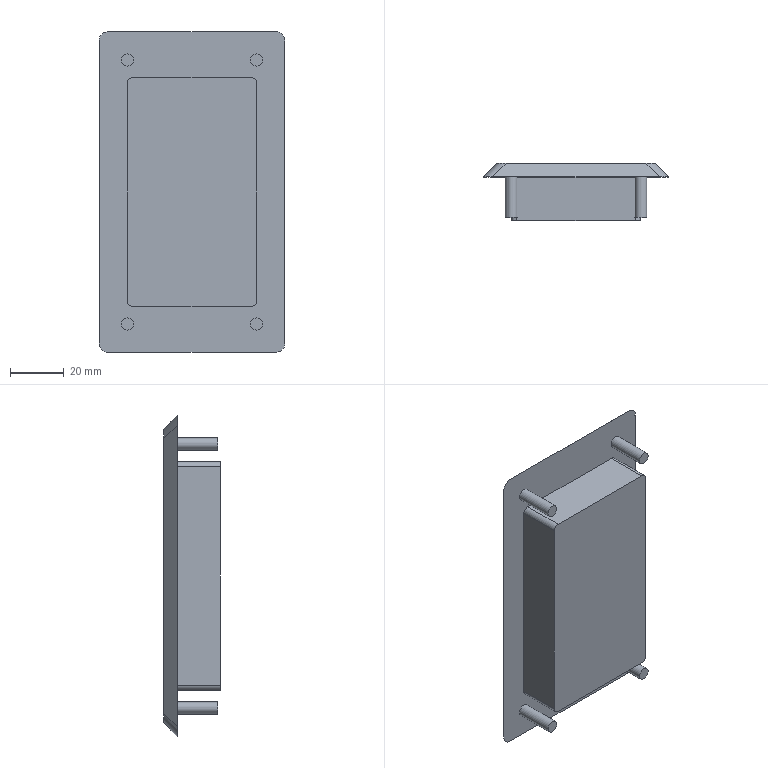Part | STEP file | 冲床-300配套压波_id522_x_t | 1 solid | 38 faces | box 69 x 21 x 119 mm | volume 44051 mm3 | plane 22 | cylinder 16 | commonest cylinder face diameters 4 x4 4.5 x4 10 x4 13 x2 20 x2
STEP:
#1=CARTESIAN_POINT('',(1655.5,280.,-353.25));
#2=VERTEX_POINT('',#1);
#3=CARTESIAN_POINT('',(1655.5,280.,-351.));
#4=DIRECTION('',(0.,-1.,0.));
#5=DIRECTION('',(0.,0.,-1.));
#6=AXIS2_PLACEMENT_3D('',#3,#4,#5);
#7=CIRCLE('',#6,2.25);
#8=EDGE_CURVE('',#2,#2,#7,.T.);
#9=ORIENTED_EDGE('',*,*,#8,.F.);
#10=EDGE_LOOP('',(#9));
#11=FACE_BOUND('',#10,.T.);
#12=CARTESIAN_POINT('',(1607.5,280.,-353.25));
#13=VERTEX_POINT('',#12);
#14=CARTESIAN_POINT('',(1607.5,280.,-351.));
#15=DIRECTION('',(0.,-1.,0.));
#16=DIRECTION('',(0.,0.,-1.));
#17=AXIS2_PLACEMENT_3D('',#14,#15,#16);
#18=CIRCLE('',#17,2.25);
#19=EDGE_CURVE('',#13,#13,#18,.T.);
#20=ORIENTED_EDGE('',*,*,#19,.F.);
#21=EDGE_LOOP('',(#20));
#22=FACE_BOUND('',#21,.T.);
#23=CARTESIAN_POINT('',(1609.5,280.,-442.5));
#24=VERTEX_POINT('',#23);
#25=CARTESIAN_POINT('',(1653.5,280.,-442.5));
#26=VERTEX_POINT('',#25);
#27=CARTESIAN_POINT('',(1467.,280.,-442.5));
#28=DIRECTION('',(1.,0.,0.));
#29=VECTOR('',#28,1.);
#30=LINE('',#27,#29);
#31=EDGE_CURVE('',#24,#26,#30,.T.);
#32=ORIENTED_EDGE('',*,*,#31,.F.);
#33=CARTESIAN_POINT('',(1607.5,280.,-440.5));
#34=VERTEX_POINT('',#33);
#35=CARTESIAN_POINT('',(1609.5,280.,-440.5));
#36=DIRECTION('',(0.,1.,0.));
#37=DIRECTION('',(0.,0.,-1.));
#38=AXIS2_PLACEMENT_3D('',#35,#36,#37);
#39=CIRCLE('',#38,2.);
#40=EDGE_CURVE('',#24,#34,#39,.T.);
#41=ORIENTED_EDGE('',*,*,#40,.T.);
#42=CARTESIAN_POINT('',(1607.5,280.,-359.5));
#43=VERTEX_POINT('',#42);
#44=CARTESIAN_POINT('',(1607.5,280.,-85.5));
#45=DIRECTION('',(0.,0.,-1.));
#46=VECTOR('',#45,1.);
#47=LINE('',#44,#46);
#48=EDGE_CURVE('',#43,#34,#47,.T.);
#49=ORIENTED_EDGE('',*,*,#48,.F.);
#50=CARTESIAN_POINT('',(1609.5,280.,-357.5));
#51=VERTEX_POINT('',#50);
#52=CARTESIAN_POINT('',(1609.5,280.,-359.5));
#53=DIRECTION('',(0.,1.,0.));
#54=DIRECTION('',(0.,0.,-1.));
#55=AXIS2_PLACEMENT_3D('',#52,#53,#54);
#56=CIRCLE('',#55,2.);
#57=EDGE_CURVE('',#43,#51,#56,.T.);
#58=ORIENTED_EDGE('',*,*,#57,.T.);
#59=CARTESIAN_POINT('',(1653.5,280.,-357.5));
#60=VERTEX_POINT('',#59);
#61=CARTESIAN_POINT('',(1467.,280.,-357.5));
#62=DIRECTION('',(-1.,0.,0.));
#63=VECTOR('',#62,1.);
#64=LINE('',#61,#63);
#65=EDGE_CURVE('',#60,#51,#64,.T.);
#66=ORIENTED_EDGE('',*,*,#65,.F.);
#67=CARTESIAN_POINT('',(1655.5,280.,-359.5));
#68=VERTEX_POINT('',#67);
#69=CARTESIAN_POINT('',(1653.5,280.,-359.5));
#70=DIRECTION('',(0.,1.,0.));
#71=DIRECTION('',(0.,0.,-1.));
#72=AXIS2_PLACEMENT_3D('',#69,#70,#71);
#73=CIRCLE('',#72,2.);
#74=EDGE_CURVE('',#60,#68,#73,.T.);
#75=ORIENTED_EDGE('',*,*,#74,.T.);
#76=CARTESIAN_POINT('',(1655.5,280.,-440.5));
#77=VERTEX_POINT('',#76);
#78=CARTESIAN_POINT('',(1655.5,280.,-85.5));
#79=DIRECTION('',(0.,0.,1.));
#80=VECTOR('',#79,1.);
#81=LINE('',#78,#80);
#82=EDGE_CURVE('',#77,#68,#81,.T.);
#83=ORIENTED_EDGE('',*,*,#82,.F.);
#84=CARTESIAN_POINT('',(1653.5,280.,-440.5));
#85=DIRECTION('',(0.,1.,0.));
#86=DIRECTION('',(0.,0.,-1.));
#87=AXIS2_PLACEMENT_3D('',#84,#85,#86);
#88=CIRCLE('',#87,2.);
#89=EDGE_CURVE('',#77,#26,#88,.T.);
#90=ORIENTED_EDGE('',*,*,#89,.T.);
#91=EDGE_LOOP('',(#32,#41,#49,#58,#66,#75,#83,#90));
#92=FACE_BOUND('',#91,.T.);
#93=CARTESIAN_POINT('',(1666.,280.,-344.036));
#94=VERTEX_POINT('',#93);
#95=CARTESIAN_POINT('',(1666.,280.,-455.964));
#96=VERTEX_POINT('',#95);
#97=CARTESIAN_POINT('',(1666.,280.,-459.5));
#98=DIRECTION('',(0.,0.,-1.));
#99=VECTOR('',#98,1.);
#100=LINE('',#97,#99);
#101=EDGE_CURVE('',#94,#96,#100,.T.);
#102=ORIENTED_EDGE('',*,*,#101,.F.);
#103=CARTESIAN_POINT('',(1662.464,280.,-340.5));
#104=VERTEX_POINT('',#103);
#105=CARTESIAN_POINT('',(1658.929,280.,-347.571));
#106=DIRECTION('',(0.,-1.,0.));
#107=DIRECTION('',(0.7071,0.,0.7071));
#108=AXIS2_PLACEMENT_3D('',#105,#106,#107);
#109=ELLIPSE('',#108,8.66,5.);
#110=EDGE_CURVE('',#94,#104,#109,.T.);
#111=ORIENTED_EDGE('',*,*,#110,.T.);
#112=CARTESIAN_POINT('',(1600.536,280.,-340.5));
#113=VERTEX_POINT('',#112);
#114=CARTESIAN_POINT('',(1666.,280.,-340.5));
#115=DIRECTION('',(1.,0.,0.));
#116=VECTOR('',#115,1.);
#117=LINE('',#114,#116);
#118=EDGE_CURVE('',#113,#104,#117,.T.);
#119=ORIENTED_EDGE('',*,*,#118,.F.);
#120=CARTESIAN_POINT('',(1597.,280.,-344.036));
#121=VERTEX_POINT('',#120);
#122=CARTESIAN_POINT('',(1604.071,280.,-347.571));
#123=DIRECTION('',(0.,-1.,0.));
#124=DIRECTION('',(-0.7071,0.,0.7071));
#125=AXIS2_PLACEMENT_3D('',#122,#123,#124);
#126=ELLIPSE('',#125,8.66,5.);
#127=EDGE_CURVE('',#113,#121,#126,.T.);
#128=ORIENTED_EDGE('',*,*,#127,.T.);
#129=CARTESIAN_POINT('',(1597.,280.,-455.964));
#130=VERTEX_POINT('',#129);
#131=CARTESIAN_POINT('',(1597.,280.,-340.5));
#132=DIRECTION('',(0.,0.,1.));
#133=VECTOR('',#132,1.);
#134=LINE('',#131,#133);
#135=EDGE_CURVE('',#130,#121,#134,.T.);
#136=ORIENTED_EDGE('',*,*,#135,.F.);
#137=CARTESIAN_POINT('',(1600.536,280.,-459.5));
#138=VERTEX_POINT('',#137);
#139=CARTESIAN_POINT('',(1604.071,280.,-452.429));
#140=DIRECTION('',(0.,-1.,0.));
#141=DIRECTION('',(-0.7071,0.,-0.7071));
#142=AXIS2_PLACEMENT_3D('',#139,#140,#141);
#143=ELLIPSE('',#142,8.66,5.);
#144=EDGE_CURVE('',#130,#138,#143,.T.);
#145=ORIENTED_EDGE('',*,*,#144,.T.);
#146=CARTESIAN_POINT('',(1662.464,280.,-459.5));
#147=VERTEX_POINT('',#146);
#148=CARTESIAN_POINT('',(1597.,280.,-459.5));
#149=DIRECTION('',(-1.,0.,0.));
#150=VECTOR('',#149,1.);
#151=LINE('',#148,#150);
#152=EDGE_CURVE('',#147,#138,#151,.T.);
#153=ORIENTED_EDGE('',*,*,#152,.F.);
#154=CARTESIAN_POINT('',(1658.929,280.,-452.429));
#155=DIRECTION('',(0.,-1.,0.));
#156=DIRECTION('',(0.7071,0.,-0.7071));
#157=AXIS2_PLACEMENT_3D('',#154,#155,#156);
#158=ELLIPSE('',#157,8.66,5.);
#159=EDGE_CURVE('',#147,#96,#158,.T.);
#160=ORIENTED_EDGE('',*,*,#159,.T.);
#161=EDGE_LOOP('',(#102,#111,#119,#128,#136,#145,#153,#160));
#162=FACE_BOUND('',#161,.T.);
#163=CARTESIAN_POINT('',(1655.5,280.,-451.25));
#164=VERTEX_POINT('',#163);
#165=CARTESIAN_POINT('',(1655.5,280.,-449.));
#166=DIRECTION('',(0.,-1.,0.));
#167=DIRECTION('',(0.,0.,-1.));
#168=AXIS2_PLACEMENT_3D('',#165,#166,#167);
#169=CIRCLE('',#168,2.25);
#170=EDGE_CURVE('',#164,#164,#169,.T.);
#171=ORIENTED_EDGE('',*,*,#170,.F.);
#172=EDGE_LOOP('',(#171));
#173=FACE_BOUND('',#172,.T.);
#174=CARTESIAN_POINT('',(1607.5,280.,-451.25));
#175=VERTEX_POINT('',#174);
#176=CARTESIAN_POINT('',(1607.5,280.,-449.));
#177=DIRECTION('',(0.,1.,0.));
#178=DIRECTION('',(0.,0.,-1.));
#179=AXIS2_PLACEMENT_3D('',#176,#177,#178);
#180=CIRCLE('',#179,2.25);
#181=EDGE_CURVE('',#175,#175,#180,.T.);
#182=ORIENTED_EDGE('',*,*,#181,.T.);
#183=EDGE_LOOP('',(#182));
#184=FACE_BOUND('',#183,.T.);
#185=CARTESIAN_POINT('',(1467.,280.,-85.5));
#186=DIRECTION('',(0.,1.,0.));
#187=DIRECTION('',(0.,0.,-1.));
#188=AXIS2_PLACEMENT_3D('',#185,#186,#187);
#189=PLANE('',#188);
#190=ADVANCED_FACE('',(#11,#22,#92,#162,#173,#184),#189,.F.);
#191=CARTESIAN_POINT('',(1648.5,285.,-359.5));
#192=VERTEX_POINT('',#191);
#193=CARTESIAN_POINT('',(1655.,285.,-366.));
#194=VERTEX_POINT('',#193);
#195=CARTESIAN_POINT('',(1648.5,285.,-366.));
#196=DIRECTION('',(0.,1.,0.));
#197=DIRECTION('',(0.,0.,-1.));
#198=AXIS2_PLACEMENT_3D('',#195,#196,#197);
#199=CIRCLE('',#198,6.5);
#200=EDGE_CURVE('',#192,#194,#199,.T.);
#201=ORIENTED_EDGE('',*,*,#200,.F.);
#202=CARTESIAN_POINT('',(1627.,285.,-359.5));
#203=VERTEX_POINT('',#202);
#204=CARTESIAN_POINT('',(1467.,285.,-359.5));
#205=DIRECTION('',(-1.,0.,0.));
#206=VECTOR('',#205,1.);
#207=LINE('',#204,#206);
#208=EDGE_CURVE('',#192,#203,#207,.T.);
#209=ORIENTED_EDGE('',*,*,#208,.T.);
#210=CARTESIAN_POINT('',(1627.,285.,-440.5));
#211=VERTEX_POINT('',#210);
#212=CARTESIAN_POINT('',(1627.,285.,-85.5));
#213=DIRECTION('',(0.,0.,-1.));
#214=VECTOR('',#213,1.);
#215=LINE('',#212,#214);
#216=EDGE_CURVE('',#203,#211,#215,.T.);
#217=ORIENTED_EDGE('',*,*,#216,.T.);
#218=CARTESIAN_POINT('',(1648.5,285.,-440.5));
#219=VERTEX_POINT('',#218);
#220=CARTESIAN_POINT('',(1467.,285.,-440.5));
#221=DIRECTION('',(1.,0.,0.));
#222=VECTOR('',#221,1.);
#223=LINE('',#220,#222);
#224=EDGE_CURVE('',#211,#219,#223,.T.);
#225=ORIENTED_EDGE('',*,*,#224,.T.);
#226=CARTESIAN_POINT('',(1655.,285.,-434.));
#227=VERTEX_POINT('',#226);
#228=CARTESIAN_POINT('',(1648.5,285.,-434.));
#229=DIRECTION('',(0.,1.,0.));
#230=DIRECTION('',(0.,0.,-1.));
#231=AXIS2_PLACEMENT_3D('',#228,#229,#230);
#232=CIRCLE('',#231,6.5);
#233=EDGE_CURVE('',#227,#219,#232,.T.);
#234=ORIENTED_EDGE('',*,*,#233,.F.);
#235=CARTESIAN_POINT('',(1655.,285.,-85.5));
#236=DIRECTION('',(0.,0.,1.));
#237=VECTOR('',#236,1.);
#238=LINE('',#235,#237);
#239=EDGE_CURVE('',#227,#194,#238,.T.);
#240=ORIENTED_EDGE('',*,*,#239,.T.);
#241=EDGE_LOOP('',(#201,#209,#217,#225,#234,#240));
#242=FACE_BOUND('',#241,.T.);
#243=CARTESIAN_POINT('',(1657.464,285.,-454.5));
#244=VERTEX_POINT('',#243);
#245=CARTESIAN_POINT('',(1605.536,285.,-454.5));
#246=VERTEX_POINT('',#245);
#247=CARTESIAN_POINT('',(1661.,285.,-454.5));
#248=DIRECTION('',(-1.,0.,0.));
#249=VECTOR('',#248,1.);
#250=LINE('',#247,#249);
#251=EDGE_CURVE('',#244,#246,#250,.T.);
#252=ORIENTED_EDGE('',*,*,#251,.T.);
#253=CARTESIAN_POINT('',(1602.,285.,-450.964));
#254=VERTEX_POINT('',#253);
#255=CARTESIAN_POINT('',(1609.071,285.,-447.429));
#256=DIRECTION('',(0.,1.,0.));
#257=DIRECTION('',(-0.7071,0.,-0.7071));
#258=AXIS2_PLACEMENT_3D('',#255,#256,#257);
#259=ELLIPSE('',#258,8.66,5.);
#260=EDGE_CURVE('',#246,#254,#259,.T.);
#261=ORIENTED_EDGE('',*,*,#260,.T.);
#262=CARTESIAN_POINT('',(1602.,285.,-349.036));
#263=VERTEX_POINT('',#262);
#264=CARTESIAN_POINT('',(1602.,285.,-454.5));
#265=DIRECTION('',(0.,0.,1.));
#266=VECTOR('',#265,1.);
#267=LINE('',#264,#266);
#268=EDGE_CURVE('',#254,#263,#267,.T.);
#269=ORIENTED_EDGE('',*,*,#268,.T.);
#270=CARTESIAN_POINT('',(1605.536,285.,-345.5));
#271=VERTEX_POINT('',#270);
#272=CARTESIAN_POINT('',(1609.071,285.,-352.571));
#273=DIRECTION('',(0.,1.,0.));
#274=DIRECTION('',(-0.7071,0.,0.7071));
#275=AXIS2_PLACEMENT_3D('',#272,#273,#274);
#276=ELLIPSE('',#275,8.66,5.);
#277=EDGE_CURVE('',#263,#271,#276,.T.);
#278=ORIENTED_EDGE('',*,*,#277,.T.);
#279=CARTESIAN_POINT('',(1657.464,285.,-345.5));
#280=VERTEX_POINT('',#279);
#281=CARTESIAN_POINT('',(1602.,285.,-345.5));
#282=DIRECTION('',(1.,0.,0.));
#283=VECTOR('',#282,1.);
#284=LINE('',#281,#283);
#285=EDGE_CURVE('',#271,#280,#284,.T.);
#286=ORIENTED_EDGE('',*,*,#285,.T.);
#287=CARTESIAN_POINT('',(1661.,285.,-349.036));
#288=VERTEX_POINT('',#287);
#289=CARTESIAN_POINT('',(1653.929,285.,-352.571));
#290=DIRECTION('',(0.,1.,0.));
#291=DIRECTION('',(0.7071,0.,0.7071));
#292=AXIS2_PLACEMENT_3D('',#289,#290,#291);
#293=ELLIPSE('',#292,8.66,5.);
#294=EDGE_CURVE('',#280,#288,#293,.T.);
#295=ORIENTED_EDGE('',*,*,#294,.T.);
#296=CARTESIAN_POINT('',(1661.,285.,-450.964));
#297=VERTEX_POINT('',#296);
#298=CARTESIAN_POINT('',(1661.,285.,-345.5));
#299=DIRECTION('',(0.,0.,-1.));
#300=VECTOR('',#299,1.);
#301=LINE('',#298,#300);
#302=EDGE_CURVE('',#288,#297,#301,.T.);
#303=ORIENTED_EDGE('',*,*,#302,.T.);
#304=CARTESIAN_POINT('',(1653.929,285.,-447.429));
#305=DIRECTION('',(0.,1.,0.));
#306=DIRECTION('',(0.7071,0.,-0.7071));
#307=AXIS2_PLACEMENT_3D('',#304,#305,#306);
#308=ELLIPSE('',#307,8.66,5.);
#309=EDGE_CURVE('',#297,#244,#308,.T.);
#310=ORIENTED_EDGE('',*,*,#309,.T.);
#311=EDGE_LOOP('',(#252,#261,#269,#278,#286,#295,#303,#310));
#312=FACE_BOUND('',#311,.T.);
#313=CARTESIAN_POINT('',(1467.,285.,-85.5));
#314=DIRECTION('',(0.,1.,0.));
#315=DIRECTION('',(0.,0.,-1.));
#316=AXIS2_PLACEMENT_3D('',#313,#314,#315);
#317=PLANE('',#316);
#318=ADVANCED_FACE('',(#242,#312),#317,.T.);
#319=CARTESIAN_POINT('',(1619.,266.5,-440.5));
#320=VERTEX_POINT('',#319);
#321=CARTESIAN_POINT('',(1648.5,266.5,-440.5));
#322=VERTEX_POINT('',#321);
#323=CARTESIAN_POINT('',(1467.,266.5,-440.5));
#324=DIRECTION('',(1.,0.,0.));
#325=VECTOR('',#324,1.);
#326=LINE('',#323,#325);
#327=EDGE_CURVE('',#320,#322,#326,.T.);
#328=ORIENTED_EDGE('',*,*,#327,.T.);
#329=CARTESIAN_POINT('',(1648.5,254.,-440.5));
#330=DIRECTION('',(0.,-1.,0.));
#331=VECTOR('',#330,1.);
#332=LINE('',#329,#331);
#333=EDGE_CURVE('',#219,#322,#332,.T.);
#334=ORIENTED_EDGE('',*,*,#333,.F.);
#335=ORIENTED_EDGE('',*,*,#224,.F.);
#336=CARTESIAN_POINT('',(1627.,278.5,-440.5));
#337=VERTEX_POINT('',#336);
#338=CARTESIAN_POINT('',(1627.,254.,-440.5));
#339=DIRECTION('',(0.,1.,0.));
#340=VECTOR('',#339,1.);
#341=LINE('',#338,#340);
#342=EDGE_CURVE('',#337,#211,#341,.T.);
#343=ORIENTED_EDGE('',*,*,#342,.F.);
#344=CARTESIAN_POINT('',(1619.,278.5,-440.5));
#345=VERTEX_POINT('',#344);
#346=CARTESIAN_POINT('',(1655.,278.5,-440.5));
#347=DIRECTION('',(-1.,0.,0.));
#348=VECTOR('',#347,1.);
#349=LINE('',#346,#348);
#350=EDGE_CURVE('',#337,#345,#349,.T.);
#351=ORIENTED_EDGE('',*,*,#350,.T.);
#352=CARTESIAN_POINT('',(1619.,254.,-440.5));
#353=DIRECTION('',(0.,-1.,0.));
#354=VECTOR('',#353,1.);
#355=LINE('',#352,#354);
#356=EDGE_CURVE('',#345,#320,#355,.T.);
#357=ORIENTED_EDGE('',*,*,#356,.T.);
#358=EDGE_LOOP('',(#328,#334,#335,#343,#351,#357));
#359=FACE_OUTER_BOUND('',#358,.T.);
#360=CARTESIAN_POINT('',(1655.,254.,-440.5));
#361=DIRECTION('',(0.,0.,1.));
#362=DIRECTION('',(1.,0.,0.));
#363=AXIS2_PLACEMENT_3D('',#360,#361,#362);
#364=PLANE('',#363);
#365=ADVANCED_FACE('',(#359),#364,.T.);
#366=CARTESIAN_POINT('',(1655.,266.5,-434.));
#367=VERTEX_POINT('',#366);
#368=CARTESIAN_POINT('',(1655.,254.,-434.));
#369=DIRECTION('',(0.,-1.,0.));
#370=VECTOR('',#369,1.);
#371=LINE('',#368,#370);
#372=EDGE_CURVE('',#227,#367,#371,.T.);
#373=ORIENTED_EDGE('',*,*,#372,.T.);
#374=CARTESIAN_POINT('',(1655.,266.5,-366.));
#375=VERTEX_POINT('',#374);
#376=CARTESIAN_POINT('',(1655.,266.5,-85.5));
#377=DIRECTION('',(0.,0.,1.));
#378=VECTOR('',#377,1.);
#379=LINE('',#376,#378);
#380=EDGE_CURVE('',#367,#375,#379,.T.);
#381=ORIENTED_EDGE('',*,*,#380,.T.);
#382=CARTESIAN_POINT('',(1655.,254.,-366.));
#383=DIRECTION('',(0.,-1.,0.));
#384=VECTOR('',#383,1.);
#385=LINE('',#382,#384);
#386=EDGE_CURVE('',#194,#375,#385,.T.);
#387=ORIENTED_EDGE('',*,*,#386,.F.);
#388=ORIENTED_EDGE('',*,*,#239,.F.);
#389=EDGE_LOOP('',(#373,#381,#387,#388));
#390=FACE_OUTER_BOUND('',#389,.T.);
#391=CARTESIAN_POINT('',(1655.,254.,-359.5));
#392=DIRECTION('',(-1.,0.,0.));
#393=DIRECTION('',(0.,0.,1.));
#394=AXIS2_PLACEMENT_3D('',#391,#392,#393);
#395=PLANE('',#394);
#396=ADVANCED_FACE('',(#390),#395,.T.);
#397=CARTESIAN_POINT('',(1619.,278.5,-359.5));
#398=VERTEX_POINT('',#397);
#399=CARTESIAN_POINT('',(1627.,278.5,-359.5));
#400=VERTEX_POINT('',#399);
#401=CARTESIAN_POINT('',(1627.,278.5,-359.5));
#402=DIRECTION('',(1.,0.,0.));
#403=VECTOR('',#402,1.);
#404=LINE('',#401,#403);
#405=EDGE_CURVE('',#398,#400,#404,.T.);
#406=ORIENTED_EDGE('',*,*,#405,.T.);
#407=CARTESIAN_POINT('',(1627.,279.,-359.5));
#408=DIRECTION('',(0.,1.,0.));
#409=VECTOR('',#408,1.);
#410=LINE('',#407,#409);
#411=EDGE_CURVE('',#400,#203,#410,.T.);
#412=ORIENTED_EDGE('',*,*,#411,.T.);
#413=ORIENTED_EDGE('',*,*,#208,.F.);
#414=CARTESIAN_POINT('',(1648.5,266.5,-359.5));
#415=VERTEX_POINT('',#414);
#416=CARTESIAN_POINT('',(1648.5,254.,-359.5));
#417=DIRECTION('',(0.,-1.,0.));
#418=VECTOR('',#417,1.);
#419=LINE('',#416,#418);
#420=EDGE_CURVE('',#192,#415,#419,.T.);
#421=ORIENTED_EDGE('',*,*,#420,.T.);
#422=CARTESIAN_POINT('',(1619.,266.5,-359.5));
#423=VERTEX_POINT('',#422);
#424=CARTESIAN_POINT('',(1467.,266.5,-359.5));
#425=DIRECTION('',(-1.,0.,0.));
#426=VECTOR('',#425,1.);
#427=LINE('',#424,#426);
#428=EDGE_CURVE('',#415,#423,#427,.T.);
#429=ORIENTED_EDGE('',*,*,#428,.T.);
#430=CARTESIAN_POINT('',(1619.,254.,-359.5));
#431=DIRECTION('',(0.,1.,0.));
#432=VECTOR('',#431,1.);
#433=LINE('',#430,#432);
#434=EDGE_CURVE('',#423,#398,#433,.T.);
#435=ORIENTED_EDGE('',*,*,#434,.T.);
#436=EDGE_LOOP('',(#406,#412,#413,#421,#429,#435));
#437=FACE_OUTER_BOUND('',#436,.T.);
#438=CARTESIAN_POINT('',(1627.,254.,-359.5));
#439=DIRECTION('',(0.,0.,-1.));
#440=DIRECTION('',(-1.,0.,0.));
#441=AXIS2_PLACEMENT_3D('',#438,#439,#440);
#442=PLANE('',#441);
#443=ADVANCED_FACE('',(#437),#442,.T.);
#444=ORIENTED_EDGE('',*,*,#342,.T.);
#445=ORIENTED_EDGE('',*,*,#216,.F.);
#446=ORIENTED_EDGE('',*,*,#411,.F.);
#447=CARTESIAN_POINT('',(1627.,278.5,-359.5));
#448=DIRECTION('',(0.,0.,-1.));
#449=VECTOR('',#448,1.);
#450=LINE('',#447,#449);
#451=EDGE_CURVE('',#400,#337,#450,.T.);
#452=ORIENTED_EDGE('',*,*,#451,.T.);
#453=EDGE_LOOP('',(#444,#445,#446,#452));
#454=FACE_OUTER_BOUND('',#453,.T.);
#455=CARTESIAN_POINT('',(1627.,279.,-359.5));
#456=DIRECTION('',(-1.,0.,0.));
#457=DIRECTION('',(0.,0.,1.));
#458=AXIS2_PLACEMENT_3D('',#455,#456,#457);
#459=PLANE('',#458);
#460=ADVANCED_FACE('',(#454),#459,.F.);
#461=CARTESIAN_POINT('',(1609.,278.5,-369.5));
#462=VERTEX_POINT('',#461);
#463=CARTESIAN_POINT('',(1609.,278.5,-430.5));
#464=VERTEX_POINT('',#463);
#465=CARTESIAN_POINT('',(1609.,278.5,-443.));
#466=DIRECTION('',(0.,0.,-1.));
#467=VECTOR('',#466,1.);
#468=LINE('',#465,#467);
#469=EDGE_CURVE('',#462,#464,#468,.T.);
#470=ORIENTED_EDGE('',*,*,#469,.F.);
#471=CARTESIAN_POINT('',(1609.,266.5,-369.5));
#472=VERTEX_POINT('',#471);
#473=CARTESIAN_POINT('',(1609.,265.,-369.5));
#474=DIRECTION('',(0.,-1.,0.));
#475=VECTOR('',#474,1.);
#476=LINE('',#473,#475);
#477=EDGE_CURVE('',#462,#472,#476,.T.);
#478=ORIENTED_EDGE('',*,*,#477,.T.);
#479=CARTESIAN_POINT('',(1609.,266.5,-430.5));
#480=VERTEX_POINT('',#479);
#481=CARTESIAN_POINT('',(1609.,266.5,-443.));
#482=DIRECTION('',(0.,0.,-1.));
#483=VECTOR('',#482,1.);
#484=LINE('',#481,#483);
#485=EDGE_CURVE('',#472,#480,#484,.T.);
#486=ORIENTED_EDGE('',*,*,#485,.T.);
#487=CARTESIAN_POINT('',(1609.,265.,-430.5));
#488=DIRECTION('',(0.,1.,0.));
#489=VECTOR('',#488,1.);
#490=LINE('',#487,#489);
#491=EDGE_CURVE('',#480,#464,#490,.T.);
#492=ORIENTED_EDGE('',*,*,#491,.T.);
#493=EDGE_LOOP('',(#470,#478,#486,#492));
#494=FACE_OUTER_BOUND('',#493,.T.);
#495=CARTESIAN_POINT('',(1609.,265.,-443.));
#496=DIRECTION('',(1.,0.,0.));
#497=DIRECTION('',(0.,0.,-1.));
#498=AXIS2_PLACEMENT_3D('',#495,#496,#497);
#499=PLANE('',#498);
#500=ADVANCED_FACE('',(#494),#499,.T.);
#501=ORIENTED_EDGE('',*,*,#485,.F.);
#502=CARTESIAN_POINT('',(1619.,266.5,-369.5));
#503=DIRECTION('',(0.,1.,0.));
#504=DIRECTION('',(0.,0.,1.));
#505=AXIS2_PLACEMENT_3D('',#502,#503,#504);
#506=CIRCLE('',#505,10.);
#507=EDGE_CURVE('',#472,#423,#506,.T.);
#508=ORIENTED_EDGE('',*,*,#507,.T.);
#509=ORIENTED_EDGE('',*,*,#428,.F.);
#510=CARTESIAN_POINT('',(1648.5,266.5,-366.));
#511=DIRECTION('',(0.,-1.,0.));
#512=DIRECTION('',(0.,0.,1.));
#513=AXIS2_PLACEMENT_3D('',#510,#511,#512);
#514=CIRCLE('',#513,6.5);
#515=EDGE_CURVE('',#375,#415,#514,.T.);
#516=ORIENTED_EDGE('',*,*,#515,.F.);
#517=ORIENTED_EDGE('',*,*,#380,.F.);
#518=CARTESIAN_POINT('',(1648.5,266.5,-434.));
#519=DIRECTION('',(0.,-1.,0.));
#520=DIRECTION('',(0.,0.,1.));
#521=AXIS2_PLACEMENT_3D('',#518,#519,#520);
#522=CIRCLE('',#521,6.5);
#523=EDGE_CURVE('',#322,#367,#522,.T.);
#524=ORIENTED_EDGE('',*,*,#523,.F.);
#525=ORIENTED_EDGE('',*,*,#327,.F.);
#526=CARTESIAN_POINT('',(1619.,266.5,-430.5));
#527=DIRECTION('',(0.,1.,0.));
#528=DIRECTION('',(0.,0.,1.));
#529=AXIS2_PLACEMENT_3D('',#526,#527,#528);
#530=CIRCLE('',#529,10.);
#531=EDGE_CURVE('',#320,#480,#530,.T.);
#532=ORIENTED_EDGE('',*,*,#531,.T.);
#533=EDGE_LOOP('',(#501,#508,#509,#516,#517,#524,#525,#532));
#534=FACE_OUTER_BOUND('',#533,.T.);
#535=CARTESIAN_POINT('',(1467.,266.5,-85.5));
#536=DIRECTION('',(0.,-1.,0.));
#537=DIRECTION('',(0.,0.,1.));
#538=AXIS2_PLACEMENT_3D('',#535,#536,#537);
#539=PLANE('',#538);
#540=ADVANCED_FACE('',(#534),#539,.F.);
#541=ORIENTED_EDGE('',*,*,#350,.F.);
#542=ORIENTED_EDGE('',*,*,#451,.F.);
#543=ORIENTED_EDGE('',*,*,#405,.F.);
#544=CARTESIAN_POINT('',(1619.,278.5,-369.5));
#545=DIRECTION('',(0.,-1.,0.));
#546=DIRECTION('',(0.,0.,1.));
#547=AXIS2_PLACEMENT_3D('',#544,#545,#546);
#548=CIRCLE('',#547,10.);
#549=EDGE_CURVE('',#398,#462,#548,.T.);
#550=ORIENTED_EDGE('',*,*,#549,.T.);
#551=ORIENTED_EDGE('',*,*,#469,.T.);
#552=CARTESIAN_POINT('',(1619.,278.5,-430.5));
#553=DIRECTION('',(0.,-1.,0.));
#554=DIRECTION('',(0.,0.,1.));
#555=AXIS2_PLACEMENT_3D('',#552,#553,#554);
#556=CIRCLE('',#555,10.);
#557=EDGE_CURVE('',#464,#345,#556,.T.);
#558=ORIENTED_EDGE('',*,*,#557,.T.);
#559=EDGE_LOOP('',(#541,#542,#543,#550,#551,#558));
#560=FACE_OUTER_BOUND('',#559,.T.);
#561=CARTESIAN_POINT('',(1467.,278.5,-85.5));
#562=DIRECTION('',(0.,-1.,0.));
#563=DIRECTION('',(0.,0.,1.));
#564=AXIS2_PLACEMENT_3D('',#561,#562,#563);
#565=PLANE('',#564);
#566=ADVANCED_FACE('',(#560),#565,.T.);
#567=ORIENTED_EDGE('',*,*,#523,.T.);
#568=ORIENTED_EDGE('',*,*,#372,.F.);
#569=ORIENTED_EDGE('',*,*,#233,.T.);
#570=ORIENTED_EDGE('',*,*,#333,.T.);
#571=EDGE_LOOP('',(#567,#568,#569,#570));
#572=FACE_OUTER_BOUND('',#571,.T.);
#573=CARTESIAN_POINT('',(1648.5,254.,-434.));
#574=DIRECTION('',(0.,1.,0.));
#575=DIRECTION('',(0.,0.,-1.));
#576=AXIS2_PLACEMENT_3D('',#573,#574,#575);
#577=CYLINDRICAL_SURFACE('',#576,6.5);
#578=ADVANCED_FACE('',(#572),#577,.F.);
#579=ORIENTED_EDGE('',*,*,#515,.T.);
#580=ORIENTED_EDGE('',*,*,#420,.F.);
#581=ORIENTED_EDGE('',*,*,#200,.T.);
#582=ORIENTED_EDGE('',*,*,#386,.T.);
#583=EDGE_LOOP('',(#579,#580,#581,#582));
#584=FACE_OUTER_BOUND('',#583,.T.);
#585=CARTESIAN_POINT('',(1648.5,254.,-366.));
#586=DIRECTION('',(0.,1.,0.));
#587=DIRECTION('',(0.,0.,-1.));
#588=AXIS2_PLACEMENT_3D('',#585,#586,#587);
#589=CYLINDRICAL_SURFACE('',#588,6.5);
#590=ADVANCED_FACE('',(#584),#589,.F.);
#591=ORIENTED_EDGE('',*,*,#118,.T.);
#592=CARTESIAN_POINT('',(1593.976,348.488,-408.988));
#593=DIRECTION('',(-0.5774,0.5774,-0.5774));
#594=VECTOR('',#593,1.);
#595=LINE('',#592,#594);
#596=EDGE_CURVE('',#104,#280,#595,.T.);
#597=ORIENTED_EDGE('',*,*,#596,.T.);
#598=ORIENTED_EDGE('',*,*,#285,.F.);
#599=CARTESIAN_POINT('',(1559.357,238.821,-299.321));
#600=DIRECTION('',(-0.5774,-0.5774,0.5774));
#601=VECTOR('',#600,1.);
#602=LINE('',#599,#601);
#603=EDGE_CURVE('',#271,#113,#602,.T.);
#604=ORIENTED_EDGE('',*,*,#603,.T.);
#605=EDGE_LOOP('',(#591,#597,#598,#604));
#606=FACE_OUTER_BOUND('',#605,.T.);
#607=CARTESIAN_POINT('',(1467.,285.,-345.5));
#608=DIRECTION('',(0.,0.7071,0.7071));
#609=DIRECTION('',(1.,0.,0.));
#610=AXIS2_PLACEMENT_3D('',#607,#608,#609);
#611=PLANE('',#610);
#612=ADVANCED_FACE('',(#606),#611,.T.);
#613=ORIENTED_EDGE('',*,*,#302,.F.);
#614=CARTESIAN_POINT('',(1748.845,197.155,-261.19));
#615=DIRECTION('',(0.5774,-0.5774,0.5774));
#616=VECTOR('',#615,1.);
#617=LINE('',#614,#616);
#618=EDGE_CURVE('',#288,#94,#617,.T.);
#619=ORIENTED_EDGE('',*,*,#618,.T.);
#620=ORIENTED_EDGE('',*,*,#101,.T.);
#621=CARTESIAN_POINT('',(1539.179,406.821,-329.143));
#622=DIRECTION('',(-0.5774,0.5774,0.5774));
#623=VECTOR('',#622,1.);
#624=LINE('',#621,#623);
#625=EDGE_CURVE('',#96,#297,#624,.T.);
#626=ORIENTED_EDGE('',*,*,#625,.T.);
#627=EDGE_LOOP('',(#613,#619,#620,#626));
#628=FACE_OUTER_BOUND('',#627,.T.);
#629=CARTESIAN_POINT('',(1661.,285.,-85.5));
#630=DIRECTION('',(0.7071,0.7071,0.));
#631=DIRECTION('',(0.,0.,-1.));
#632=AXIS2_PLACEMENT_3D('',#629,#630,#631);
#633=PLANE('',#632);
#634=ADVANCED_FACE('',(#628),#633,.T.);
#635=ORIENTED_EDGE('',*,*,#135,.T.);
#636=CARTESIAN_POINT('',(1514.155,197.155,-261.19));
#637=DIRECTION('',(0.5774,0.5774,-0.5774));
#638=VECTOR('',#637,1.);
#639=LINE('',#636,#638);
#640=EDGE_CURVE('',#121,#263,#639,.T.);
#641=ORIENTED_EDGE('',*,*,#640,.T.);
#642=ORIENTED_EDGE('',*,*,#268,.F.);
#643=CARTESIAN_POINT('',(1723.821,406.821,-329.143));
#644=DIRECTION('',(-0.5774,-0.5774,-0.5774));
#645=VECTOR('',#644,1.);
#646=LINE('',#643,#645);
#647=EDGE_CURVE('',#254,#130,#646,.T.);
#648=ORIENTED_EDGE('',*,*,#647,.T.);
#649=EDGE_LOOP('',(#635,#641,#642,#648));
#650=FACE_OUTER_BOUND('',#649,.T.);
#651=CARTESIAN_POINT('',(1602.,285.,-85.5));
#652=DIRECTION('',(-0.7071,0.7071,0.));
#653=DIRECTION('',(0.,0.,1.));
#654=AXIS2_PLACEMENT_3D('',#651,#652,#653);
#655=PLANE('',#654);
#656=ADVANCED_FACE('',(#650),#655,.T.);
#657=ORIENTED_EDGE('',*,*,#152,.T.);
#658=CARTESIAN_POINT('',(1559.357,238.821,-500.679));
#659=DIRECTION('',(0.5774,0.5774,0.5774));
#660=VECTOR('',#659,1.);
#661=LINE('',#658,#660);
#662=EDGE_CURVE('',#138,#246,#661,.T.);
#663=ORIENTED_EDGE('',*,*,#662,.T.);
#664=ORIENTED_EDGE('',*,*,#251,.F.);
#665=CARTESIAN_POINT('',(1593.976,348.488,-391.012));
#666=DIRECTION('',(0.5774,-0.5774,-0.5774));
#667=VECTOR('',#666,1.);
#668=LINE('',#665,#667);
#669=EDGE_CURVE('',#244,#147,#668,.T.);
#670=ORIENTED_EDGE('',*,*,#669,.T.);
#671=EDGE_LOOP('',(#657,#663,#664,#670));
#672=FACE_OUTER_BOUND('',#671,.T.);
#673=CARTESIAN_POINT('',(1467.,285.,-454.5));
#674=DIRECTION('',(0.,0.7071,-0.7071));
#675=DIRECTION('',(-1.,0.,0.));
#676=AXIS2_PLACEMENT_3D('',#673,#674,#675);
#677=PLANE('',#676);
#678=ADVANCED_FACE('',(#672),#677,.T.);
#679=ORIENTED_EDGE('',*,*,#309,.F.);
#680=ORIENTED_EDGE('',*,*,#625,.F.);
#681=ORIENTED_EDGE('',*,*,#159,.F.);
#682=ORIENTED_EDGE('',*,*,#669,.F.);
#683=EDGE_LOOP('',(#679,#680,#681,#682));
#684=FACE_OUTER_BOUND('',#683,.T.);
#685=CARTESIAN_POINT('',(1535.643,403.286,-329.143));
#686=DIRECTION('',(0.5774,-0.5774,-0.5774));
#687=DIRECTION('',(-0.7071,0.,-0.7071));
#688=AXIS2_PLACEMENT_3D('',#685,#686,#687);
#689=CYLINDRICAL_SURFACE('',#688,5.);
#690=ADVANCED_FACE('',(#684),#689,.T.);
#691=ORIENTED_EDGE('',*,*,#260,.F.);
#692=ORIENTED_EDGE('',*,*,#662,.F.);
#693=ORIENTED_EDGE('',*,*,#144,.F.);
#694=ORIENTED_EDGE('',*,*,#647,.F.);
#695=EDGE_LOOP('',(#691,#692,#693,#694));
#696=FACE_OUTER_BOUND('',#695,.T.);
#697=CARTESIAN_POINT('',(1559.357,235.286,-497.143));
#698=DIRECTION('',(-0.5774,-0.5774,-0.5774));
#699=DIRECTION('',(-0.7071,0.,0.7071));
#700=AXIS2_PLACEMENT_3D('',#697,#698,#699);
#701=CYLINDRICAL_SURFACE('',#700,5.);
#702=ADVANCED_FACE('',(#696),#701,.T.);
#703=ORIENTED_EDGE('',*,*,#277,.F.);
#704=ORIENTED_EDGE('',*,*,#640,.F.);
#705=ORIENTED_EDGE('',*,*,#127,.F.);
#706=ORIENTED_EDGE('',*,*,#603,.F.);
#707=EDGE_LOOP('',(#703,#704,#705,#706));
#708=FACE_OUTER_BOUND('',#707,.T.);
#709=CARTESIAN_POINT('',(1517.69,193.619,-261.19));
#710=DIRECTION('',(-0.5774,-0.5774,0.5774));
#711=DIRECTION('',(0.7071,0.,0.7071));
#712=AXIS2_PLACEMENT_3D('',#709,#710,#711);
#713=CYLINDRICAL_SURFACE('',#712,5.);
#714=ADVANCED_FACE('',(#708),#713,.T.);
#715=ORIENTED_EDGE('',*,*,#294,.F.);
#716=ORIENTED_EDGE('',*,*,#596,.F.);
#717=ORIENTED_EDGE('',*,*,#110,.F.);
#718=ORIENTED_EDGE('',*,*,#618,.F.);
#719=EDGE_LOOP('',(#715,#716,#717,#718));
#720=FACE_OUTER_BOUND('',#719,.T.);
#721=CARTESIAN_POINT('',(1593.976,344.953,-412.524));
#722=DIRECTION('',(0.5774,-0.5774,0.5774));
#723=DIRECTION('',(0.7071,0.,-0.7071));
#724=AXIS2_PLACEMENT_3D('',#721,#722,#723);
#725=CYLINDRICAL_SURFACE('',#724,5.);
#726=ADVANCED_FACE('',(#720),#725,.T.);
#727=CARTESIAN_POINT('',(1655.5,264.,-440.5));
#728=VERTEX_POINT('',#727);
#729=CARTESIAN_POINT('',(1655.5,264.,-359.5));
#730=VERTEX_POINT('',#729);
#731=CARTESIAN_POINT('',(1655.5,264.,-357.));
#732=DIRECTION('',(0.,0.,1.));
#733=VECTOR('',#732,1.);
#734=LINE('',#731,#733);
#735=EDGE_CURVE('',#728,#730,#734,.T.);
#736=ORIENTED_EDGE('',*,*,#735,.T.);
#737=CARTESIAN_POINT('',(1653.5,264.,-357.5));
#738=VERTEX_POINT('',#737);
#739=CARTESIAN_POINT('',(1653.5,264.,-359.5));
#740=DIRECTION('',(0.,-1.,0.));
#741=DIRECTION('',(0.,0.,1.));
#742=AXIS2_PLACEMENT_3D('',#739,#740,#741);
#743=CIRCLE('',#742,2.);
#744=EDGE_CURVE('',#730,#738,#743,.T.);
#745=ORIENTED_EDGE('',*,*,#744,.T.);
#746=CARTESIAN_POINT('',(1609.5,264.,-357.5));
#747=VERTEX_POINT('',#746);
#748=CARTESIAN_POINT('',(1605.,264.,-357.5));
#749=DIRECTION('',(-1.,0.,0.));
#750=VECTOR('',#749,1.);
#751=LINE('',#748,#750);
#752=EDGE_CURVE('',#738,#747,#751,.T.);
#753=ORIENTED_EDGE('',*,*,#752,.T.);
#754=CARTESIAN_POINT('',(1607.5,264.,-359.5));
#755=VERTEX_POINT('',#754);
#756=CARTESIAN_POINT('',(1609.5,264.,-359.5));
#757=DIRECTION('',(0.,-1.,0.));
#758=DIRECTION('',(0.,0.,1.));
#759=AXIS2_PLACEMENT_3D('',#756,#757,#758);
#760=CIRCLE('',#759,2.);
#761=EDGE_CURVE('',#747,#755,#760,.T.);
#762=ORIENTED_EDGE('',*,*,#761,.T.);
#763=CARTESIAN_POINT('',(1607.5,264.,-440.5));
#764=VERTEX_POINT('',#763);
#765=CARTESIAN_POINT('',(1607.5,264.,-443.));
#766=DIRECTION('',(0.,0.,-1.));
#767=VECTOR('',#766,1.);
#768=LINE('',#765,#767);
#769=EDGE_CURVE('',#755,#764,#768,.T.);
#770=ORIENTED_EDGE('',*,*,#769,.T.);
#771=CARTESIAN_POINT('',(1609.5,264.,-442.5));
#772=VERTEX_POINT('',#771);
#773=CARTESIAN_POINT('',(1609.5,264.,-440.5));
#774=DIRECTION('',(0.,-1.,0.));
#775=DIRECTION('',(0.,0.,1.));
#776=AXIS2_PLACEMENT_3D('',#773,#774,#775);
#777=CIRCLE('',#776,2.);
#778=EDGE_CURVE('',#764,#772,#777,.T.);
#779=ORIENTED_EDGE('',*,*,#778,.T.);
#780=CARTESIAN_POINT('',(1653.5,264.,-442.5));
#781=VERTEX_POINT('',#780);
#782=CARTESIAN_POINT('',(1658.,264.,-442.5));
#783=DIRECTION('',(1.,0.,0.));
#784=VECTOR('',#783,1.);
#785=LINE('',#782,#784);
#786=EDGE_CURVE('',#772,#781,#785,.T.);
#787=ORIENTED_EDGE('',*,*,#786,.T.);
#788=CARTESIAN_POINT('',(1653.5,264.,-440.5));
#789=DIRECTION('',(0.,-1.,0.));
#790=DIRECTION('',(0.,0.,1.));
#791=AXIS2_PLACEMENT_3D('',#788,#789,#790);
#792=CIRCLE('',#791,2.);
#793=EDGE_CURVE('',#781,#728,#792,.T.);
#794=ORIENTED_EDGE('',*,*,#793,.T.);
#795=EDGE_LOOP('',(#736,#745,#753,#762,#770,#779,#787,#794));
#796=FACE_OUTER_BOUND('',#795,.T.);
#797=CARTESIAN_POINT('',(1467.,264.,-85.5));
#798=DIRECTION('',(0.,-1.,0.));
#799=DIRECTION('',(0.,0.,1.));
#800=AXIS2_PLACEMENT_3D('',#797,#798,#799);
#801=PLANE('',#800);
#802=ADVANCED_FACE('',(#796),#801,.T.);
#803=ORIENTED_EDGE('',*,*,#786,.F.);
#804=CARTESIAN_POINT('',(1609.5,265.,-442.5));
#805=DIRECTION('',(0.,1.,0.));
#806=VECTOR('',#805,1.);
#807=LINE('',#804,#806);
#808=EDGE_CURVE('',#772,#24,#807,.T.);
#809=ORIENTED_EDGE('',*,*,#808,.T.);
#810=ORIENTED_EDGE('',*,*,#31,.T.);
#811=CARTESIAN_POINT('',(1653.5,265.,-442.5));
#812=DIRECTION('',(0.,-1.,0.));
#813=VECTOR('',#812,1.);
#814=LINE('',#811,#813);
#815=EDGE_CURVE('',#26,#781,#814,.T.);
#816=ORIENTED_EDGE('',*,*,#815,.T.);
#817=EDGE_LOOP('',(#803,#809,#810,#816));
#818=FACE_OUTER_BOUND('',#817,.T.);
#819=CARTESIAN_POINT('',(1658.,265.,-442.5));
#820=DIRECTION('',(0.,0.,1.));
#821=DIRECTION('',(1.,0.,0.));
#822=AXIS2_PLACEMENT_3D('',#819,#820,#821);
#823=PLANE('',#822);
#824=ADVANCED_FACE('',(#818),#823,.F.);
#825=ORIENTED_EDGE('',*,*,#48,.T.);
#826=CARTESIAN_POINT('',(1607.5,265.,-440.5));
#827=DIRECTION('',(0.,-1.,0.));
#828=VECTOR('',#827,1.);
#829=LINE('',#826,#828);
#830=EDGE_CURVE('',#34,#764,#829,.T.);
#831=ORIENTED_EDGE('',*,*,#830,.T.);
#832=ORIENTED_EDGE('',*,*,#769,.F.);
#833=CARTESIAN_POINT('',(1607.5,265.,-359.5));
#834=DIRECTION('',(0.,1.,0.));
#835=VECTOR('',#834,1.);
#836=LINE('',#833,#835);
#837=EDGE_CURVE('',#755,#43,#836,.T.);
#838=ORIENTED_EDGE('',*,*,#837,.T.);
#839=EDGE_LOOP('',(#825,#831,#832,#838));
#840=FACE_OUTER_BOUND('',#839,.T.);
#841=CARTESIAN_POINT('',(1607.5,265.,-443.));
#842=DIRECTION('',(1.,0.,0.));
#843=DIRECTION('',(0.,0.,-1.));
#844=AXIS2_PLACEMENT_3D('',#841,#842,#843);
#845=PLANE('',#844);
#846=ADVANCED_FACE('',(#840),#845,.F.);
#847=ORIENTED_EDGE('',*,*,#65,.T.);
#848=CARTESIAN_POINT('',(1609.5,265.,-357.5));
#849=DIRECTION('',(0.,-1.,0.));
#850=VECTOR('',#849,1.);
#851=LINE('',#848,#850);
#852=EDGE_CURVE('',#51,#747,#851,.T.);
#853=ORIENTED_EDGE('',*,*,#852,.T.);
#854=ORIENTED_EDGE('',*,*,#752,.F.);
#855=CARTESIAN_POINT('',(1653.5,265.,-357.5));
#856=DIRECTION('',(0.,1.,0.));
#857=VECTOR('',#856,1.);
#858=LINE('',#855,#857);
#859=EDGE_CURVE('',#738,#60,#858,.T.);
#860=ORIENTED_EDGE('',*,*,#859,.T.);
#861=EDGE_LOOP('',(#847,#853,#854,#860));
#862=FACE_OUTER_BOUND('',#861,.T.);
#863=CARTESIAN_POINT('',(1605.,265.,-357.5));
#864=DIRECTION('',(0.,0.,-1.));
#865=DIRECTION('',(-1.,0.,0.));
#866=AXIS2_PLACEMENT_3D('',#863,#864,#865);
#867=PLANE('',#866);
#868=ADVANCED_FACE('',(#862),#867,.F.);
#869=ORIENTED_EDGE('',*,*,#82,.T.);
#870=CARTESIAN_POINT('',(1655.5,265.,-359.5));
#871=DIRECTION('',(0.,-1.,0.));
#872=VECTOR('',#871,1.);
#873=LINE('',#870,#872);
#874=EDGE_CURVE('',#68,#730,#873,.T.);
#875=ORIENTED_EDGE('',*,*,#874,.T.);
#876=ORIENTED_EDGE('',*,*,#735,.F.);
#877=CARTESIAN_POINT('',(1655.5,265.,-440.5));
#878=DIRECTION('',(0.,1.,0.));
#879=VECTOR('',#878,1.);
#880=LINE('',#877,#879);
#881=EDGE_CURVE('',#728,#77,#880,.T.);
#882=ORIENTED_EDGE('',*,*,#881,.T.);
#883=EDGE_LOOP('',(#869,#875,#876,#882));
#884=FACE_OUTER_BOUND('',#883,.T.);
#885=CARTESIAN_POINT('',(1655.5,265.,-357.));
#886=DIRECTION('',(-1.,0.,0.));
#887=DIRECTION('',(0.,0.,1.));
#888=AXIS2_PLACEMENT_3D('',#885,#886,#887);
#889=PLANE('',#888);
#890=ADVANCED_FACE('',(#884),#889,.F.);
#891=CARTESIAN_POINT('',(1607.5,265.,-451.25));
#892=VERTEX_POINT('',#891);
#893=CARTESIAN_POINT('',(1607.5,265.,-449.));
#894=DIRECTION('',(0.,1.,0.));
#895=DIRECTION('',(0.,0.,-1.));
#896=AXIS2_PLACEMENT_3D('',#893,#894,#895);
#897=CIRCLE('',#896,2.25);
#898=EDGE_CURVE('',#892,#892,#897,.T.);
#899=ORIENTED_EDGE('',*,*,#898,.T.);
#900=EDGE_LOOP('',(#899));
#901=FACE_BOUND('',#900,.T.);
#902=ORIENTED_EDGE('',*,*,#181,.F.);
#903=EDGE_LOOP('',(#902));
#904=FACE_BOUND('',#903,.T.);
#905=CARTESIAN_POINT('',(1607.5,260.,-449.));
#906=DIRECTION('',(0.,1.,0.));
#907=DIRECTION('',(0.,0.,-1.));
#908=AXIS2_PLACEMENT_3D('',#905,#906,#907);
#909=CYLINDRICAL_SURFACE('',#908,2.25);
#910=ADVANCED_FACE('',(#901,#904),#909,.T.);
#911=ORIENTED_EDGE('',*,*,#898,.F.);
#912=EDGE_LOOP('',(#911));
#913=FACE_OUTER_BOUND('',#912,.T.);
#914=CARTESIAN_POINT('',(1607.5,265.,-449.));
#915=DIRECTION('',(0.,1.,0.));
#916=DIRECTION('',(0.,0.,-1.));
#917=AXIS2_PLACEMENT_3D('',#914,#915,#916);
#918=PLANE('',#917);
#919=ADVANCED_FACE('',(#913),#918,.F.);
#920=CARTESIAN_POINT('',(1655.5,265.,-348.75));
#921=VERTEX_POINT('',#920);
#922=CARTESIAN_POINT('',(1655.5,265.,-351.));
#923=DIRECTION('',(0.,-1.,0.));
#924=DIRECTION('',(0.,0.,1.));
#925=AXIS2_PLACEMENT_3D('',#922,#923,#924);
#926=CIRCLE('',#925,2.25);
#927=EDGE_CURVE('',#921,#921,#926,.T.);
#928=ORIENTED_EDGE('',*,*,#927,.F.);
#929=EDGE_LOOP('',(#928));
#930=FACE_BOUND('',#929,.T.);
#931=ORIENTED_EDGE('',*,*,#8,.T.);
#932=EDGE_LOOP('',(#931));
#933=FACE_BOUND('',#932,.T.);
#934=CARTESIAN_POINT('',(1655.5,260.,-351.));
#935=DIRECTION('',(0.,1.,0.));
#936=DIRECTION('',(0.,0.,-1.));
#937=AXIS2_PLACEMENT_3D('',#934,#935,#936);
#938=CYLINDRICAL_SURFACE('',#937,2.25);
#939=ADVANCED_FACE('',(#930,#933),#938,.T.);
#940=ORIENTED_EDGE('',*,*,#927,.T.);
#941=EDGE_LOOP('',(#940));
#942=FACE_OUTER_BOUND('',#941,.T.);
#943=CARTESIAN_POINT('',(1655.5,265.,-351.));
#944=DIRECTION('',(0.,-1.,0.));
#945=DIRECTION('',(0.,0.,1.));
#946=AXIS2_PLACEMENT_3D('',#943,#944,#945);
#947=PLANE('',#946);
#948=ADVANCED_FACE('',(#942),#947,.T.);
#949=CARTESIAN_POINT('',(1655.5,265.,-446.75));
#950=VERTEX_POINT('',#949);
#951=CARTESIAN_POINT('',(1655.5,265.,-449.));
#952=DIRECTION('',(0.,-1.,0.));
#953=DIRECTION('',(0.,0.,1.));
#954=AXIS2_PLACEMENT_3D('',#951,#952,#953);
#955=CIRCLE('',#954,2.25);
#956=EDGE_CURVE('',#950,#950,#955,.T.);
#957=ORIENTED_EDGE('',*,*,#956,.F.);
#958=EDGE_LOOP('',(#957));
#959=FACE_BOUND('',#958,.T.);
#960=ORIENTED_EDGE('',*,*,#170,.T.);
#961=EDGE_LOOP('',(#960));
#962=FACE_BOUND('',#961,.T.);
#963=CARTESIAN_POINT('',(1655.5,260.,-449.));
#964=DIRECTION('',(0.,1.,0.));
#965=DIRECTION('',(0.,0.,-1.));
#966=AXIS2_PLACEMENT_3D('',#963,#964,#965);
#967=CYLINDRICAL_SURFACE('',#966,2.25);
#968=ADVANCED_FACE('',(#959,#962),#967,.T.);
#969=ORIENTED_EDGE('',*,*,#956,.T.);
#970=EDGE_LOOP('',(#969));
#971=FACE_OUTER_BOUND('',#970,.T.);
#972=CARTESIAN_POINT('',(1655.5,265.,-449.));
#973=DIRECTION('',(0.,-1.,0.));
#974=DIRECTION('',(0.,0.,1.));
#975=AXIS2_PLACEMENT_3D('',#972,#973,#974);
#976=PLANE('',#975);
#977=ADVANCED_FACE('',(#971),#976,.T.);
#978=ORIENTED_EDGE('',*,*,#19,.T.);
#979=EDGE_LOOP('',(#978));
#980=FACE_BOUND('',#979,.T.);
#981=CARTESIAN_POINT('',(1607.5,265.,-353.25));
#982=VERTEX_POINT('',#981);
#983=CARTESIAN_POINT('',(1607.5,265.,-351.));
#984=DIRECTION('',(0.,1.,0.));
#985=DIRECTION('',(0.,0.,-1.));
#986=AXIS2_PLACEMENT_3D('',#983,#984,#985);
#987=CIRCLE('',#986,2.25);
#988=EDGE_CURVE('',#982,#982,#987,.T.);
#989=ORIENTED_EDGE('',*,*,#988,.T.);
#990=EDGE_LOOP('',(#989));
#991=FACE_BOUND('',#990,.T.);
#992=CARTESIAN_POINT('',(1607.5,260.,-351.));
#993=DIRECTION('',(0.,1.,0.));
#994=DIRECTION('',(0.,0.,-1.));
#995=AXIS2_PLACEMENT_3D('',#992,#993,#994);
#996=CYLINDRICAL_SURFACE('',#995,2.25);
#997=ADVANCED_FACE('',(#980,#991),#996,.T.);
#998=ORIENTED_EDGE('',*,*,#988,.F.);
#999=EDGE_LOOP('',(#998));
#1000=FACE_OUTER_BOUND('',#999,.T.);
#1001=CARTESIAN_POINT('',(1607.5,265.,-351.));
#1002=DIRECTION('',(0.,1.,0.));
#1003=DIRECTION('',(0.,0.,-1.));
#1004=AXIS2_PLACEMENT_3D('',#1001,#1002,#1003);
#1005=PLANE('',#1004);
#1006=ADVANCED_FACE('',(#1000),#1005,.F.);
#1007=ORIENTED_EDGE('',*,*,#557,.F.);
#1008=ORIENTED_EDGE('',*,*,#491,.F.);
#1009=ORIENTED_EDGE('',*,*,#531,.F.);
#1010=ORIENTED_EDGE('',*,*,#356,.F.);
#1011=EDGE_LOOP('',(#1007,#1008,#1009,#1010));
#1012=FACE_OUTER_BOUND('',#1011,.T.);
#1013=CARTESIAN_POINT('',(1619.,265.,-430.5));
#1014=DIRECTION('',(0.,1.,0.));
#1015=DIRECTION('',(0.,0.,-1.));
#1016=AXIS2_PLACEMENT_3D('',#1013,#1014,#1015);
#1017=CYLINDRICAL_SURFACE('',#1016,10.);
#1018=ADVANCED_FACE('',(#1012),#1017,.F.);
#1019=ORIENTED_EDGE('',*,*,#549,.F.);
#1020=ORIENTED_EDGE('',*,*,#434,.F.);
#1021=ORIENTED_EDGE('',*,*,#507,.F.);
#1022=ORIENTED_EDGE('',*,*,#477,.F.);
#1023=EDGE_LOOP('',(#1019,#1020,#1021,#1022));
#1024=FACE_OUTER_BOUND('',#1023,.T.);
#1025=CARTESIAN_POINT('',(1619.,254.,-369.5));
#1026=DIRECTION('',(0.,1.,0.));
#1027=DIRECTION('',(0.,0.,-1.));
#1028=AXIS2_PLACEMENT_3D('',#1025,#1026,#1027);
#1029=CYLINDRICAL_SURFACE('',#1028,10.);
#1030=ADVANCED_FACE('',(#1024),#1029,.F.);
#1031=ORIENTED_EDGE('',*,*,#793,.F.);
#1032=ORIENTED_EDGE('',*,*,#815,.F.);
#1033=ORIENTED_EDGE('',*,*,#89,.F.);
#1034=ORIENTED_EDGE('',*,*,#881,.F.);
#1035=EDGE_LOOP('',(#1031,#1032,#1033,#1034));
#1036=FACE_OUTER_BOUND('',#1035,.T.);
#1037=CARTESIAN_POINT('',(1653.5,265.,-440.5));
#1038=DIRECTION('',(0.,1.,0.));
#1039=DIRECTION('',(0.,0.,-1.));
#1040=AXIS2_PLACEMENT_3D('',#1037,#1038,#1039);
#1041=CYLINDRICAL_SURFACE('',#1040,2.);
#1042=ADVANCED_FACE('',(#1036),#1041,.T.);
#1043=ORIENTED_EDGE('',*,*,#744,.F.);
#1044=ORIENTED_EDGE('',*,*,#874,.F.);
#1045=ORIENTED_EDGE('',*,*,#74,.F.);
#1046=ORIENTED_EDGE('',*,*,#859,.F.);
#1047=EDGE_LOOP('',(#1043,#1044,#1045,#1046));
#1048=FACE_OUTER_BOUND('',#1047,.T.);
#1049=CARTESIAN_POINT('',(1653.5,265.,-359.5));
#1050=DIRECTION('',(0.,1.,0.));
#1051=DIRECTION('',(0.,0.,-1.));
#1052=AXIS2_PLACEMENT_3D('',#1049,#1050,#1051);
#1053=CYLINDRICAL_SURFACE('',#1052,2.);
#1054=ADVANCED_FACE('',(#1048),#1053,.T.);
#1055=ORIENTED_EDGE('',*,*,#761,.F.);
#1056=ORIENTED_EDGE('',*,*,#852,.F.);
#1057=ORIENTED_EDGE('',*,*,#57,.F.);
#1058=ORIENTED_EDGE('',*,*,#837,.F.);
#1059=EDGE_LOOP('',(#1055,#1056,#1057,#1058));
#1060=FACE_OUTER_BOUND('',#1059,.T.);
#1061=CARTESIAN_POINT('',(1609.5,265.,-359.5));
#1062=DIRECTION('',(0.,1.,0.));
#1063=DIRECTION('',(0.,0.,-1.));
#1064=AXIS2_PLACEMENT_3D('',#1061,#1062,#1063);
#1065=CYLINDRICAL_SURFACE('',#1064,2.);
#1066=ADVANCED_FACE('',(#1060),#1065,.T.);
#1067=ORIENTED_EDGE('',*,*,#778,.F.);
#1068=ORIENTED_EDGE('',*,*,#830,.F.);
#1069=ORIENTED_EDGE('',*,*,#40,.F.);
#1070=ORIENTED_EDGE('',*,*,#808,.F.);
#1071=EDGE_LOOP('',(#1067,#1068,#1069,#1070));
#1072=FACE_OUTER_BOUND('',#1071,.T.);
#1073=CARTESIAN_POINT('',(1609.5,265.,-440.5));
#1074=DIRECTION('',(0.,1.,0.));
#1075=DIRECTION('',(0.,0.,-1.));
#1076=AXIS2_PLACEMENT_3D('',#1073,#1074,#1075);
#1077=CYLINDRICAL_SURFACE('',#1076,2.);
#1078=ADVANCED_FACE('',(#1072),#1077,.T.);
#1079=CLOSED_SHELL('',(#190,#318,#365,#396,#443,#460,#500,#540,#566,#578,#590,#612,#634,#656,#678,#690,#702,#714,#726,#802,#824,#846,#868,#890,#910,#919,#939,#948,#968,#977,#997,#1006,#1018,#1030,#1042,#1054,#1066,#1078));
#1080=MANIFOLD_SOLID_BREP('',#1079);
#1081=(LENGTH_UNIT()NAMED_UNIT(*)SI_UNIT(.MILLI.,.METRE.));
#1082=UNCERTAINTY_MEASURE_WITH_UNIT(LENGTH_MEASURE(0.00002),#1081,'','');
#1083=(NAMED_UNIT(*)PLANE_ANGLE_UNIT()SI_UNIT($,.RADIAN.));
#1084=PLANE_ANGLE_MEASURE_WITH_UNIT(PLANE_ANGLE_MEASURE(0.01745),#1083);
#1085=DIMENSIONAL_EXPONENTS(0.,0.,0.,0.,0.,0.,0.);
#1086=(CONVERSION_BASED_UNIT('DEGREE',#1084)NAMED_UNIT(#1085)PLANE_ANGLE_UNIT());
#1087=(NAMED_UNIT(*)SI_UNIT($,.STERADIAN.)SOLID_ANGLE_UNIT());
#1088=(GEOMETRIC_REPRESENTATION_CONTEXT(3)GLOBAL_UNCERTAINTY_ASSIGNED_CONTEXT((#1082))GLOBAL_UNIT_ASSIGNED_CONTEXT((#1081,#1086,#1087))REPRESENTATION_CONTEXT('',''));
#1089=ADVANCED_BREP_SHAPE_REPRESENTATION('',(#1080),#1088);